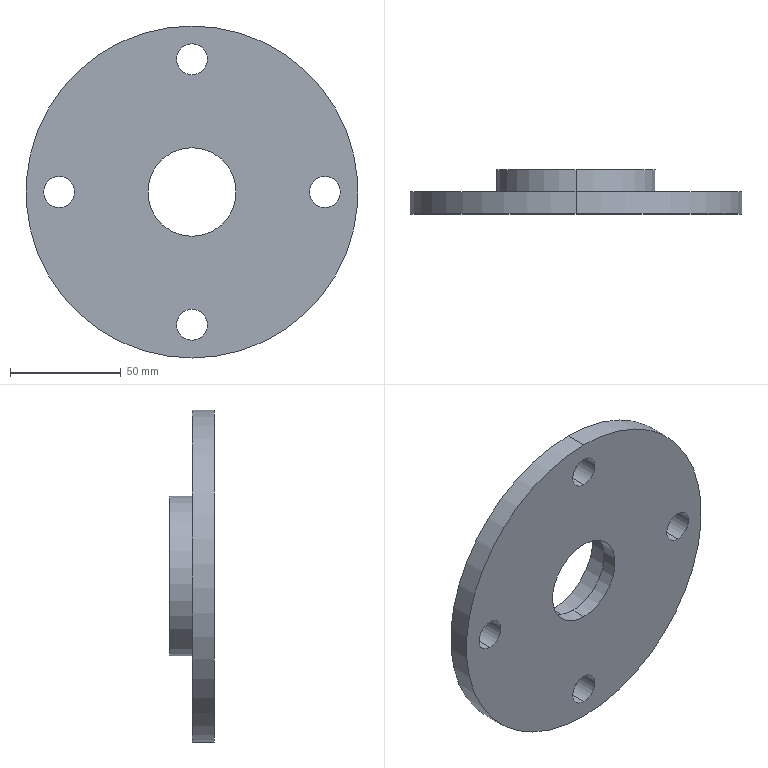Part | SolidWorks | features BaseBody 1 | 1 solid | 20 faces | box 150 x 20 x 150 mm | volume 174867 mm3 | cylinder 16 | plane 4 | commonest cylinder face diameters 14 x8 40 x2 52 x2 72 x2 150 x2
STEP:
#1=CARTESIAN_POINT('',(0.,10.,-75.));
#2=VERTEX_POINT('',#1);
#3=CARTESIAN_POINT('',(0.,10.,75.));
#4=VERTEX_POINT('',#3);
#5=CARTESIAN_POINT('',(0.,10.,0.));
#6=DIRECTION('',(0.,-1.,0.));
#7=DIRECTION('',(0.,0.,-1.));
#8=AXIS2_PLACEMENT_3D('',#5,#6,#7);
#9=CIRCLE('',#8,75.);
#10=EDGE_CURVE('',#2,#4,#9,.T.);
#11=ORIENTED_EDGE('',*,*,#10,.T.);
#12=CARTESIAN_POINT('',(0.,0.,75.));
#13=VERTEX_POINT('',#12);
#14=CARTESIAN_POINT('',(0.,10.,75.));
#15=DIRECTION('',(0.,-1.,0.));
#16=VECTOR('',#15,1000.);
#17=LINE('',#14,#16);
#18=EDGE_CURVE('',#4,#13,#17,.T.);
#19=ORIENTED_EDGE('',*,*,#18,.T.);
#20=CARTESIAN_POINT('',(0.,0.,-75.));
#21=VERTEX_POINT('',#20);
#22=CARTESIAN_POINT('',(0.,0.,0.));
#23=DIRECTION('',(0.,1.,0.));
#24=DIRECTION('',(0.,0.,-1.));
#25=AXIS2_PLACEMENT_3D('',#22,#23,#24);
#26=CIRCLE('',#25,75.);
#27=EDGE_CURVE('',#13,#21,#26,.T.);
#28=ORIENTED_EDGE('',*,*,#27,.T.);
#29=CARTESIAN_POINT('',(0.,10.,-75.));
#30=DIRECTION('',(0.,-1.,0.));
#31=VECTOR('',#30,1000.);
#32=LINE('',#29,#31);
#33=EDGE_CURVE('',#2,#21,#32,.T.);
#34=ORIENTED_EDGE('',*,*,#33,.F.);
#35=EDGE_LOOP('',(#11,#19,#28,#34));
#36=FACE_OUTER_BOUND('',#35,.T.);
#37=CARTESIAN_POINT('',(0.,10.,0.));
#38=DIRECTION('',(0.,-1.,0.));
#39=DIRECTION('',(0.,0.,-1.));
#40=AXIS2_PLACEMENT_3D('',#37,#38,#39);
#41=CYLINDRICAL_SURFACE('',#40,75.);
#42=ADVANCED_FACE('',(#36),#41,.T.);
#43=CARTESIAN_POINT('',(0.,0.,20.));
#44=VERTEX_POINT('',#43);
#45=CARTESIAN_POINT('',(0.,0.,-20.));
#46=VERTEX_POINT('',#45);
#47=CARTESIAN_POINT('',(0.,0.,0.));
#48=DIRECTION('',(0.,-1.,0.));
#49=DIRECTION('',(0.,0.,1.));
#50=AXIS2_PLACEMENT_3D('',#47,#48,#49);
#51=CIRCLE('',#50,20.);
#52=EDGE_CURVE('',#44,#46,#51,.T.);
#53=ORIENTED_EDGE('',*,*,#52,.T.);
#54=CARTESIAN_POINT('',(0.,7.,-20.));
#55=VERTEX_POINT('',#54);
#56=CARTESIAN_POINT('',(0.,0.,-20.));
#57=DIRECTION('',(0.,1.,0.));
#58=VECTOR('',#57,1000.);
#59=LINE('',#56,#58);
#60=EDGE_CURVE('',#46,#55,#59,.T.);
#61=ORIENTED_EDGE('',*,*,#60,.T.);
#62=CARTESIAN_POINT('',(0.,7.,20.));
#63=VERTEX_POINT('',#62);
#64=CARTESIAN_POINT('',(0.,7.,0.));
#65=DIRECTION('',(0.,-1.,0.));
#66=DIRECTION('',(0.,0.,1.));
#67=AXIS2_PLACEMENT_3D('',#64,#65,#66);
#68=CIRCLE('',#67,20.);
#69=EDGE_CURVE('',#63,#55,#68,.T.);
#70=ORIENTED_EDGE('',*,*,#69,.F.);
#71=CARTESIAN_POINT('',(0.,0.,20.));
#72=DIRECTION('',(0.,1.,0.));
#73=VECTOR('',#72,1000.);
#74=LINE('',#71,#73);
#75=EDGE_CURVE('',#44,#63,#74,.T.);
#76=ORIENTED_EDGE('',*,*,#75,.F.);
#77=EDGE_LOOP('',(#53,#61,#70,#76));
#78=FACE_OUTER_BOUND('',#77,.T.);
#79=CARTESIAN_POINT('',(0.,0.,0.));
#80=DIRECTION('',(0.,1.,0.));
#81=DIRECTION('',(0.,0.,1.));
#82=AXIS2_PLACEMENT_3D('',#79,#80,#81);
#83=CYLINDRICAL_SURFACE('',#82,20.);
#84=ADVANCED_FACE('',(#78),#83,.F.);
#85=CARTESIAN_POINT('',(0.,0.,-53.));
#86=VERTEX_POINT('',#85);
#87=CARTESIAN_POINT('',(0.,0.,-67.));
#88=VERTEX_POINT('',#87);
#89=CARTESIAN_POINT('',(0.,0.,-60.));
#90=DIRECTION('',(0.,-1.,0.));
#91=DIRECTION('',(0.,0.,1.));
#92=AXIS2_PLACEMENT_3D('',#89,#90,#91);
#93=CIRCLE('',#92,7.);
#94=EDGE_CURVE('',#86,#88,#93,.T.);
#95=ORIENTED_EDGE('',*,*,#94,.T.);
#96=CARTESIAN_POINT('',(0.,10.,-67.));
#97=VERTEX_POINT('',#96);
#98=CARTESIAN_POINT('',(0.,-3.,-67.));
#99=DIRECTION('',(0.,1.,0.));
#100=VECTOR('',#99,1000.);
#101=LINE('',#98,#100);
#102=EDGE_CURVE('',#88,#97,#101,.T.);
#103=ORIENTED_EDGE('',*,*,#102,.T.);
#104=CARTESIAN_POINT('',(0.,10.,-53.));
#105=VERTEX_POINT('',#104);
#106=CARTESIAN_POINT('',(0.,10.,-60.));
#107=DIRECTION('',(0.,-1.,0.));
#108=DIRECTION('',(0.,0.,1.));
#109=AXIS2_PLACEMENT_3D('',#106,#107,#108);
#110=CIRCLE('',#109,7.);
#111=EDGE_CURVE('',#105,#97,#110,.T.);
#112=ORIENTED_EDGE('',*,*,#111,.F.);
#113=CARTESIAN_POINT('',(0.,-3.,-53.));
#114=DIRECTION('',(0.,1.,0.));
#115=VECTOR('',#114,1000.);
#116=LINE('',#113,#115);
#117=EDGE_CURVE('',#86,#105,#116,.T.);
#118=ORIENTED_EDGE('',*,*,#117,.F.);
#119=EDGE_LOOP('',(#95,#103,#112,#118));
#120=FACE_OUTER_BOUND('',#119,.T.);
#121=CARTESIAN_POINT('',(0.,-3.,-60.));
#122=DIRECTION('',(0.,1.,0.));
#123=DIRECTION('',(0.,0.,1.));
#124=AXIS2_PLACEMENT_3D('',#121,#122,#123);
#125=CYLINDRICAL_SURFACE('',#124,7.);
#126=ADVANCED_FACE('',(#120),#125,.F.);
#127=CARTESIAN_POINT('',(60.,0.,7.));
#128=VERTEX_POINT('',#127);
#129=CARTESIAN_POINT('',(60.,0.,-7.));
#130=VERTEX_POINT('',#129);
#131=CARTESIAN_POINT('',(60.,0.,0.));
#132=DIRECTION('',(0.,-1.,0.));
#133=DIRECTION('',(0.,0.,1.));
#134=AXIS2_PLACEMENT_3D('',#131,#132,#133);
#135=CIRCLE('',#134,7.);
#136=EDGE_CURVE('',#128,#130,#135,.T.);
#137=ORIENTED_EDGE('',*,*,#136,.T.);
#138=CARTESIAN_POINT('',(60.,10.,-7.));
#139=VERTEX_POINT('',#138);
#140=CARTESIAN_POINT('',(60.,-3.,-7.));
#141=DIRECTION('',(0.,1.,0.));
#142=VECTOR('',#141,1000.);
#143=LINE('',#140,#142);
#144=EDGE_CURVE('',#130,#139,#143,.T.);
#145=ORIENTED_EDGE('',*,*,#144,.T.);
#146=CARTESIAN_POINT('',(60.,10.,7.));
#147=VERTEX_POINT('',#146);
#148=CARTESIAN_POINT('',(60.,10.,0.));
#149=DIRECTION('',(0.,-1.,0.));
#150=DIRECTION('',(0.,0.,1.));
#151=AXIS2_PLACEMENT_3D('',#148,#149,#150);
#152=CIRCLE('',#151,7.);
#153=EDGE_CURVE('',#147,#139,#152,.T.);
#154=ORIENTED_EDGE('',*,*,#153,.F.);
#155=CARTESIAN_POINT('',(60.,-3.,7.));
#156=DIRECTION('',(0.,1.,0.));
#157=VECTOR('',#156,1000.);
#158=LINE('',#155,#157);
#159=EDGE_CURVE('',#128,#147,#158,.T.);
#160=ORIENTED_EDGE('',*,*,#159,.F.);
#161=EDGE_LOOP('',(#137,#145,#154,#160));
#162=FACE_OUTER_BOUND('',#161,.T.);
#163=CARTESIAN_POINT('',(60.,-3.,0.));
#164=DIRECTION('',(0.,1.,0.));
#165=DIRECTION('',(0.,0.,1.));
#166=AXIS2_PLACEMENT_3D('',#163,#164,#165);
#167=CYLINDRICAL_SURFACE('',#166,7.);
#168=ADVANCED_FACE('',(#162),#167,.F.);
#169=CARTESIAN_POINT('',(0.,0.,67.));
#170=VERTEX_POINT('',#169);
#171=CARTESIAN_POINT('',(0.,0.,53.));
#172=VERTEX_POINT('',#171);
#173=CARTESIAN_POINT('',(0.,0.,60.));
#174=DIRECTION('',(0.,-1.,0.));
#175=DIRECTION('',(0.,0.,1.));
#176=AXIS2_PLACEMENT_3D('',#173,#174,#175);
#177=CIRCLE('',#176,7.);
#178=EDGE_CURVE('',#170,#172,#177,.T.);
#179=ORIENTED_EDGE('',*,*,#178,.T.);
#180=CARTESIAN_POINT('',(0.,10.,53.));
#181=VERTEX_POINT('',#180);
#182=CARTESIAN_POINT('',(0.,-3.,53.));
#183=DIRECTION('',(0.,1.,0.));
#184=VECTOR('',#183,1000.);
#185=LINE('',#182,#184);
#186=EDGE_CURVE('',#172,#181,#185,.T.);
#187=ORIENTED_EDGE('',*,*,#186,.T.);
#188=CARTESIAN_POINT('',(0.,10.,67.));
#189=VERTEX_POINT('',#188);
#190=CARTESIAN_POINT('',(0.,10.,60.));
#191=DIRECTION('',(0.,-1.,0.));
#192=DIRECTION('',(0.,0.,1.));
#193=AXIS2_PLACEMENT_3D('',#190,#191,#192);
#194=CIRCLE('',#193,7.);
#195=EDGE_CURVE('',#189,#181,#194,.T.);
#196=ORIENTED_EDGE('',*,*,#195,.F.);
#197=CARTESIAN_POINT('',(0.,-3.,67.));
#198=DIRECTION('',(0.,1.,0.));
#199=VECTOR('',#198,1000.);
#200=LINE('',#197,#199);
#201=EDGE_CURVE('',#170,#189,#200,.T.);
#202=ORIENTED_EDGE('',*,*,#201,.F.);
#203=EDGE_LOOP('',(#179,#187,#196,#202));
#204=FACE_OUTER_BOUND('',#203,.T.);
#205=CARTESIAN_POINT('',(0.,-3.,60.));
#206=DIRECTION('',(0.,1.,0.));
#207=DIRECTION('',(0.,0.,1.));
#208=AXIS2_PLACEMENT_3D('',#205,#206,#207);
#209=CYLINDRICAL_SURFACE('',#208,7.);
#210=ADVANCED_FACE('',(#204),#209,.F.);
#211=CARTESIAN_POINT('',(-60.,0.,7.));
#212=VERTEX_POINT('',#211);
#213=CARTESIAN_POINT('',(-60.,0.,-7.));
#214=VERTEX_POINT('',#213);
#215=CARTESIAN_POINT('',(-60.,0.,0.));
#216=DIRECTION('',(0.,-1.,0.));
#217=DIRECTION('',(0.,0.,1.));
#218=AXIS2_PLACEMENT_3D('',#215,#216,#217);
#219=CIRCLE('',#218,7.);
#220=EDGE_CURVE('',#212,#214,#219,.T.);
#221=ORIENTED_EDGE('',*,*,#220,.T.);
#222=CARTESIAN_POINT('',(-60.,10.,-7.));
#223=VERTEX_POINT('',#222);
#224=CARTESIAN_POINT('',(-60.,-3.,-7.));
#225=DIRECTION('',(0.,1.,0.));
#226=VECTOR('',#225,1000.);
#227=LINE('',#224,#226);
#228=EDGE_CURVE('',#214,#223,#227,.T.);
#229=ORIENTED_EDGE('',*,*,#228,.T.);
#230=CARTESIAN_POINT('',(-60.,10.,7.));
#231=VERTEX_POINT('',#230);
#232=CARTESIAN_POINT('',(-60.,10.,0.));
#233=DIRECTION('',(0.,-1.,0.));
#234=DIRECTION('',(0.,0.,1.));
#235=AXIS2_PLACEMENT_3D('',#232,#233,#234);
#236=CIRCLE('',#235,7.);
#237=EDGE_CURVE('',#231,#223,#236,.T.);
#238=ORIENTED_EDGE('',*,*,#237,.F.);
#239=CARTESIAN_POINT('',(-60.,-3.,7.));
#240=DIRECTION('',(0.,1.,0.));
#241=VECTOR('',#240,1000.);
#242=LINE('',#239,#241);
#243=EDGE_CURVE('',#212,#231,#242,.T.);
#244=ORIENTED_EDGE('',*,*,#243,.F.);
#245=EDGE_LOOP('',(#221,#229,#238,#244));
#246=FACE_OUTER_BOUND('',#245,.T.);
#247=CARTESIAN_POINT('',(-60.,-3.,0.));
#248=DIRECTION('',(0.,1.,0.));
#249=DIRECTION('',(0.,0.,1.));
#250=AXIS2_PLACEMENT_3D('',#247,#248,#249);
#251=CYLINDRICAL_SURFACE('',#250,7.);
#252=ADVANCED_FACE('',(#246),#251,.F.);
#253=CARTESIAN_POINT('',(0.,20.,-36.));
#254=VERTEX_POINT('',#253);
#255=CARTESIAN_POINT('',(0.,20.,36.));
#256=VERTEX_POINT('',#255);
#257=CARTESIAN_POINT('',(0.,20.,0.));
#258=DIRECTION('',(0.,-1.,0.));
#259=DIRECTION('',(0.,0.,-1.));
#260=AXIS2_PLACEMENT_3D('',#257,#258,#259);
#261=CIRCLE('',#260,36.);
#262=EDGE_CURVE('',#254,#256,#261,.T.);
#263=ORIENTED_EDGE('',*,*,#262,.T.);
#264=CARTESIAN_POINT('',(0.,10.,36.));
#265=VERTEX_POINT('',#264);
#266=CARTESIAN_POINT('',(0.,20.,36.));
#267=DIRECTION('',(0.,-1.,0.));
#268=VECTOR('',#267,1000.);
#269=LINE('',#266,#268);
#270=EDGE_CURVE('',#256,#265,#269,.T.);
#271=ORIENTED_EDGE('',*,*,#270,.T.);
#272=CARTESIAN_POINT('',(0.,10.,-36.));
#273=VERTEX_POINT('',#272);
#274=CARTESIAN_POINT('',(0.,10.,0.));
#275=DIRECTION('',(0.,-1.,0.));
#276=DIRECTION('',(0.,0.,-1.));
#277=AXIS2_PLACEMENT_3D('',#274,#275,#276);
#278=CIRCLE('',#277,36.);
#279=EDGE_CURVE('',#273,#265,#278,.T.);
#280=ORIENTED_EDGE('',*,*,#279,.F.);
#281=CARTESIAN_POINT('',(0.,20.,-36.));
#282=DIRECTION('',(0.,-1.,0.));
#283=VECTOR('',#282,1000.);
#284=LINE('',#281,#283);
#285=EDGE_CURVE('',#254,#273,#284,.T.);
#286=ORIENTED_EDGE('',*,*,#285,.F.);
#287=EDGE_LOOP('',(#263,#271,#280,#286));
#288=FACE_OUTER_BOUND('',#287,.T.);
#289=CARTESIAN_POINT('',(0.,20.,0.));
#290=DIRECTION('',(0.,-1.,0.));
#291=DIRECTION('',(0.,0.,-1.));
#292=AXIS2_PLACEMENT_3D('',#289,#290,#291);
#293=CYLINDRICAL_SURFACE('',#292,36.);
#294=ADVANCED_FACE('',(#288),#293,.T.);
#295=CARTESIAN_POINT('',(0.,7.,-26.));
#296=VERTEX_POINT('',#295);
#297=CARTESIAN_POINT('',(0.,7.,26.));
#298=VERTEX_POINT('',#297);
#299=CARTESIAN_POINT('',(0.,7.,0.));
#300=DIRECTION('',(0.,1.,0.));
#301=DIRECTION('',(0.,0.,1.));
#302=AXIS2_PLACEMENT_3D('',#299,#300,#301);
#303=CIRCLE('',#302,26.);
#304=EDGE_CURVE('',#296,#298,#303,.T.);
#305=ORIENTED_EDGE('',*,*,#304,.F.);
#306=CARTESIAN_POINT('',(0.,20.,-26.));
#307=VERTEX_POINT('',#306);
#308=CARTESIAN_POINT('',(0.,7.,-26.));
#309=DIRECTION('',(0.,1.,0.));
#310=VECTOR('',#309,1000.);
#311=LINE('',#308,#310);
#312=EDGE_CURVE('',#296,#307,#311,.T.);
#313=ORIENTED_EDGE('',*,*,#312,.T.);
#314=CARTESIAN_POINT('',(0.,20.,26.));
#315=VERTEX_POINT('',#314);
#316=CARTESIAN_POINT('',(0.,20.,0.));
#317=DIRECTION('',(0.,-1.,0.));
#318=DIRECTION('',(0.,0.,1.));
#319=AXIS2_PLACEMENT_3D('',#316,#317,#318);
#320=CIRCLE('',#319,26.);
#321=EDGE_CURVE('',#315,#307,#320,.T.);
#322=ORIENTED_EDGE('',*,*,#321,.F.);
#323=CARTESIAN_POINT('',(0.,7.,26.));
#324=DIRECTION('',(0.,1.,0.));
#325=VECTOR('',#324,1000.);
#326=LINE('',#323,#325);
#327=EDGE_CURVE('',#298,#315,#326,.T.);
#328=ORIENTED_EDGE('',*,*,#327,.F.);
#329=EDGE_LOOP('',(#305,#313,#322,#328));
#330=FACE_OUTER_BOUND('',#329,.T.);
#331=CARTESIAN_POINT('',(0.,7.,0.));
#332=DIRECTION('',(0.,1.,0.));
#333=DIRECTION('',(0.,0.,1.));
#334=AXIS2_PLACEMENT_3D('',#331,#332,#333);
#335=CYLINDRICAL_SURFACE('',#334,26.);
#336=ADVANCED_FACE('',(#330),#335,.F.);
#337=CARTESIAN_POINT('',(0.,0.,0.));
#338=DIRECTION('',(0.,1.,0.));
#339=DIRECTION('',(0.,0.,-1.));
#340=AXIS2_PLACEMENT_3D('',#337,#338,#339);
#341=CIRCLE('',#340,75.);
#342=EDGE_CURVE('',#21,#13,#341,.T.);
#343=ORIENTED_EDGE('',*,*,#342,.F.);
#344=ORIENTED_EDGE('',*,*,#27,.F.);
#345=EDGE_LOOP('',(#343,#344));
#346=FACE_OUTER_BOUND('',#345,.T.);
#347=ORIENTED_EDGE('',*,*,#52,.F.);
#348=CARTESIAN_POINT('',(0.,0.,0.));
#349=DIRECTION('',(0.,-1.,0.));
#350=DIRECTION('',(0.,0.,1.));
#351=AXIS2_PLACEMENT_3D('',#348,#349,#350);
#352=CIRCLE('',#351,20.);
#353=EDGE_CURVE('',#46,#44,#352,.T.);
#354=ORIENTED_EDGE('',*,*,#353,.F.);
#355=EDGE_LOOP('',(#347,#354));
#356=FACE_BOUND('',#355,.T.);
#357=ORIENTED_EDGE('',*,*,#94,.F.);
#358=CARTESIAN_POINT('',(0.,0.,-60.));
#359=DIRECTION('',(0.,-1.,0.));
#360=DIRECTION('',(0.,0.,1.));
#361=AXIS2_PLACEMENT_3D('',#358,#359,#360);
#362=CIRCLE('',#361,7.);
#363=EDGE_CURVE('',#88,#86,#362,.T.);
#364=ORIENTED_EDGE('',*,*,#363,.F.);
#365=EDGE_LOOP('',(#357,#364));
#366=FACE_BOUND('',#365,.T.);
#367=ORIENTED_EDGE('',*,*,#136,.F.);
#368=CARTESIAN_POINT('',(60.,0.,0.));
#369=DIRECTION('',(0.,-1.,0.));
#370=DIRECTION('',(0.,0.,1.));
#371=AXIS2_PLACEMENT_3D('',#368,#369,#370);
#372=CIRCLE('',#371,7.);
#373=EDGE_CURVE('',#130,#128,#372,.T.);
#374=ORIENTED_EDGE('',*,*,#373,.F.);
#375=EDGE_LOOP('',(#367,#374));
#376=FACE_BOUND('',#375,.T.);
#377=ORIENTED_EDGE('',*,*,#178,.F.);
#378=CARTESIAN_POINT('',(0.,0.,60.));
#379=DIRECTION('',(0.,-1.,0.));
#380=DIRECTION('',(0.,0.,1.));
#381=AXIS2_PLACEMENT_3D('',#378,#379,#380);
#382=CIRCLE('',#381,7.);
#383=EDGE_CURVE('',#172,#170,#382,.T.);
#384=ORIENTED_EDGE('',*,*,#383,.F.);
#385=EDGE_LOOP('',(#377,#384));
#386=FACE_BOUND('',#385,.T.);
#387=ORIENTED_EDGE('',*,*,#220,.F.);
#388=CARTESIAN_POINT('',(-60.,0.,0.));
#389=DIRECTION('',(0.,-1.,0.));
#390=DIRECTION('',(0.,0.,1.));
#391=AXIS2_PLACEMENT_3D('',#388,#389,#390);
#392=CIRCLE('',#391,7.);
#393=EDGE_CURVE('',#214,#212,#392,.T.);
#394=ORIENTED_EDGE('',*,*,#393,.F.);
#395=EDGE_LOOP('',(#387,#394));
#396=FACE_BOUND('',#395,.T.);
#397=CARTESIAN_POINT('',(0.,0.,0.));
#398=DIRECTION('',(0.,1.,0.));
#399=DIRECTION('',(0.,0.,1.));
#400=AXIS2_PLACEMENT_3D('',#397,#398,#399);
#401=PLANE('',#400);
#402=ADVANCED_FACE('',(#346,#356,#366,#376,#386,#396),#401,.F.);
#403=ORIENTED_EDGE('',*,*,#18,.F.);
#404=CARTESIAN_POINT('',(0.,10.,0.));
#405=DIRECTION('',(0.,-1.,0.));
#406=DIRECTION('',(0.,0.,-1.));
#407=AXIS2_PLACEMENT_3D('',#404,#405,#406);
#408=CIRCLE('',#407,75.);
#409=EDGE_CURVE('',#4,#2,#408,.T.);
#410=ORIENTED_EDGE('',*,*,#409,.T.);
#411=ORIENTED_EDGE('',*,*,#33,.T.);
#412=ORIENTED_EDGE('',*,*,#342,.T.);
#413=EDGE_LOOP('',(#403,#410,#411,#412));
#414=FACE_OUTER_BOUND('',#413,.T.);
#415=CARTESIAN_POINT('',(0.,10.,0.));
#416=DIRECTION('',(0.,-1.,0.));
#417=DIRECTION('',(0.,0.,-1.));
#418=AXIS2_PLACEMENT_3D('',#415,#416,#417);
#419=CYLINDRICAL_SURFACE('',#418,75.);
#420=ADVANCED_FACE('',(#414),#419,.T.);
#421=ORIENTED_EDGE('',*,*,#60,.F.);
#422=ORIENTED_EDGE('',*,*,#353,.T.);
#423=ORIENTED_EDGE('',*,*,#75,.T.);
#424=CARTESIAN_POINT('',(0.,7.,0.));
#425=DIRECTION('',(0.,-1.,0.));
#426=DIRECTION('',(0.,0.,1.));
#427=AXIS2_PLACEMENT_3D('',#424,#425,#426);
#428=CIRCLE('',#427,20.);
#429=EDGE_CURVE('',#55,#63,#428,.T.);
#430=ORIENTED_EDGE('',*,*,#429,.F.);
#431=EDGE_LOOP('',(#421,#422,#423,#430));
#432=FACE_OUTER_BOUND('',#431,.T.);
#433=CARTESIAN_POINT('',(0.,0.,0.));
#434=DIRECTION('',(0.,1.,0.));
#435=DIRECTION('',(0.,0.,1.));
#436=AXIS2_PLACEMENT_3D('',#433,#434,#435);
#437=CYLINDRICAL_SURFACE('',#436,20.);
#438=ADVANCED_FACE('',(#432),#437,.F.);
#439=ORIENTED_EDGE('',*,*,#102,.F.);
#440=ORIENTED_EDGE('',*,*,#363,.T.);
#441=ORIENTED_EDGE('',*,*,#117,.T.);
#442=CARTESIAN_POINT('',(0.,10.,-60.));
#443=DIRECTION('',(0.,-1.,0.));
#444=DIRECTION('',(0.,0.,1.));
#445=AXIS2_PLACEMENT_3D('',#442,#443,#444);
#446=CIRCLE('',#445,7.);
#447=EDGE_CURVE('',#97,#105,#446,.T.);
#448=ORIENTED_EDGE('',*,*,#447,.F.);
#449=EDGE_LOOP('',(#439,#440,#441,#448));
#450=FACE_OUTER_BOUND('',#449,.T.);
#451=CARTESIAN_POINT('',(0.,-3.,-60.));
#452=DIRECTION('',(0.,1.,0.));
#453=DIRECTION('',(0.,0.,1.));
#454=AXIS2_PLACEMENT_3D('',#451,#452,#453);
#455=CYLINDRICAL_SURFACE('',#454,7.);
#456=ADVANCED_FACE('',(#450),#455,.F.);
#457=ORIENTED_EDGE('',*,*,#144,.F.);
#458=ORIENTED_EDGE('',*,*,#373,.T.);
#459=ORIENTED_EDGE('',*,*,#159,.T.);
#460=CARTESIAN_POINT('',(60.,10.,0.));
#461=DIRECTION('',(0.,-1.,0.));
#462=DIRECTION('',(0.,0.,1.));
#463=AXIS2_PLACEMENT_3D('',#460,#461,#462);
#464=CIRCLE('',#463,7.);
#465=EDGE_CURVE('',#139,#147,#464,.T.);
#466=ORIENTED_EDGE('',*,*,#465,.F.);
#467=EDGE_LOOP('',(#457,#458,#459,#466));
#468=FACE_OUTER_BOUND('',#467,.T.);
#469=CARTESIAN_POINT('',(60.,-3.,0.));
#470=DIRECTION('',(0.,1.,0.));
#471=DIRECTION('',(0.,0.,1.));
#472=AXIS2_PLACEMENT_3D('',#469,#470,#471);
#473=CYLINDRICAL_SURFACE('',#472,7.);
#474=ADVANCED_FACE('',(#468),#473,.F.);
#475=ORIENTED_EDGE('',*,*,#186,.F.);
#476=ORIENTED_EDGE('',*,*,#383,.T.);
#477=ORIENTED_EDGE('',*,*,#201,.T.);
#478=CARTESIAN_POINT('',(0.,10.,60.));
#479=DIRECTION('',(0.,-1.,0.));
#480=DIRECTION('',(0.,0.,1.));
#481=AXIS2_PLACEMENT_3D('',#478,#479,#480);
#482=CIRCLE('',#481,7.);
#483=EDGE_CURVE('',#181,#189,#482,.T.);
#484=ORIENTED_EDGE('',*,*,#483,.F.);
#485=EDGE_LOOP('',(#475,#476,#477,#484));
#486=FACE_OUTER_BOUND('',#485,.T.);
#487=CARTESIAN_POINT('',(0.,-3.,60.));
#488=DIRECTION('',(0.,1.,0.));
#489=DIRECTION('',(0.,0.,1.));
#490=AXIS2_PLACEMENT_3D('',#487,#488,#489);
#491=CYLINDRICAL_SURFACE('',#490,7.);
#492=ADVANCED_FACE('',(#486),#491,.F.);
#493=ORIENTED_EDGE('',*,*,#228,.F.);
#494=ORIENTED_EDGE('',*,*,#393,.T.);
#495=ORIENTED_EDGE('',*,*,#243,.T.);
#496=CARTESIAN_POINT('',(-60.,10.,0.));
#497=DIRECTION('',(0.,-1.,0.));
#498=DIRECTION('',(0.,0.,1.));
#499=AXIS2_PLACEMENT_3D('',#496,#497,#498);
#500=CIRCLE('',#499,7.);
#501=EDGE_CURVE('',#223,#231,#500,.T.);
#502=ORIENTED_EDGE('',*,*,#501,.F.);
#503=EDGE_LOOP('',(#493,#494,#495,#502));
#504=FACE_OUTER_BOUND('',#503,.T.);
#505=CARTESIAN_POINT('',(-60.,-3.,0.));
#506=DIRECTION('',(0.,1.,0.));
#507=DIRECTION('',(0.,0.,1.));
#508=AXIS2_PLACEMENT_3D('',#505,#506,#507);
#509=CYLINDRICAL_SURFACE('',#508,7.);
#510=ADVANCED_FACE('',(#504),#509,.F.);
#511=ORIENTED_EDGE('',*,*,#10,.F.);
#512=ORIENTED_EDGE('',*,*,#409,.F.);
#513=EDGE_LOOP('',(#511,#512));
#514=FACE_OUTER_BOUND('',#513,.T.);
#515=ORIENTED_EDGE('',*,*,#279,.T.);
#516=CARTESIAN_POINT('',(0.,10.,0.));
#517=DIRECTION('',(0.,-1.,0.));
#518=DIRECTION('',(0.,0.,-1.));
#519=AXIS2_PLACEMENT_3D('',#516,#517,#518);
#520=CIRCLE('',#519,36.);
#521=EDGE_CURVE('',#265,#273,#520,.T.);
#522=ORIENTED_EDGE('',*,*,#521,.T.);
#523=EDGE_LOOP('',(#515,#522));
#524=FACE_BOUND('',#523,.T.);
#525=ORIENTED_EDGE('',*,*,#111,.T.);
#526=ORIENTED_EDGE('',*,*,#447,.T.);
#527=EDGE_LOOP('',(#525,#526));
#528=FACE_BOUND('',#527,.T.);
#529=ORIENTED_EDGE('',*,*,#153,.T.);
#530=ORIENTED_EDGE('',*,*,#465,.T.);
#531=EDGE_LOOP('',(#529,#530));
#532=FACE_BOUND('',#531,.T.);
#533=ORIENTED_EDGE('',*,*,#195,.T.);
#534=ORIENTED_EDGE('',*,*,#483,.T.);
#535=EDGE_LOOP('',(#533,#534));
#536=FACE_BOUND('',#535,.T.);
#537=ORIENTED_EDGE('',*,*,#237,.T.);
#538=ORIENTED_EDGE('',*,*,#501,.T.);
#539=EDGE_LOOP('',(#537,#538));
#540=FACE_BOUND('',#539,.T.);
#541=CARTESIAN_POINT('',(0.,10.,0.));
#542=DIRECTION('',(0.,1.,0.));
#543=DIRECTION('',(0.,0.,1.));
#544=AXIS2_PLACEMENT_3D('',#541,#542,#543);
#545=PLANE('',#544);
#546=ADVANCED_FACE('',(#514,#524,#528,#532,#536,#540),#545,.T.);
#547=ORIENTED_EDGE('',*,*,#69,.T.);
#548=ORIENTED_EDGE('',*,*,#429,.T.);
#549=EDGE_LOOP('',(#547,#548));
#550=FACE_BOUND('',#549,.T.);
#551=CARTESIAN_POINT('',(0.,7.,0.));
#552=DIRECTION('',(0.,1.,0.));
#553=DIRECTION('',(0.,0.,1.));
#554=AXIS2_PLACEMENT_3D('',#551,#552,#553);
#555=CIRCLE('',#554,26.);
#556=EDGE_CURVE('',#298,#296,#555,.T.);
#557=ORIENTED_EDGE('',*,*,#556,.T.);
#558=ORIENTED_EDGE('',*,*,#304,.T.);
#559=EDGE_LOOP('',(#557,#558));
#560=FACE_OUTER_BOUND('',#559,.T.);
#561=CARTESIAN_POINT('',(0.,7.,0.));
#562=DIRECTION('',(0.,1.,0.));
#563=DIRECTION('',(0.,0.,1.));
#564=AXIS2_PLACEMENT_3D('',#561,#562,#563);
#565=PLANE('',#564);
#566=ADVANCED_FACE('',(#550,#560),#565,.T.);
#567=ORIENTED_EDGE('',*,*,#270,.F.);
#568=CARTESIAN_POINT('',(0.,20.,0.));
#569=DIRECTION('',(0.,-1.,0.));
#570=DIRECTION('',(0.,0.,-1.));
#571=AXIS2_PLACEMENT_3D('',#568,#569,#570);
#572=CIRCLE('',#571,36.);
#573=EDGE_CURVE('',#256,#254,#572,.T.);
#574=ORIENTED_EDGE('',*,*,#573,.T.);
#575=ORIENTED_EDGE('',*,*,#285,.T.);
#576=ORIENTED_EDGE('',*,*,#521,.F.);
#577=EDGE_LOOP('',(#567,#574,#575,#576));
#578=FACE_OUTER_BOUND('',#577,.T.);
#579=CARTESIAN_POINT('',(0.,20.,0.));
#580=DIRECTION('',(0.,-1.,0.));
#581=DIRECTION('',(0.,0.,-1.));
#582=AXIS2_PLACEMENT_3D('',#579,#580,#581);
#583=CYLINDRICAL_SURFACE('',#582,36.);
#584=ADVANCED_FACE('',(#578),#583,.T.);
#585=ORIENTED_EDGE('',*,*,#312,.F.);
#586=ORIENTED_EDGE('',*,*,#556,.F.);
#587=ORIENTED_EDGE('',*,*,#327,.T.);
#588=CARTESIAN_POINT('',(0.,20.,0.));
#589=DIRECTION('',(0.,-1.,0.));
#590=DIRECTION('',(0.,0.,1.));
#591=AXIS2_PLACEMENT_3D('',#588,#589,#590);
#592=CIRCLE('',#591,26.);
#593=EDGE_CURVE('',#307,#315,#592,.T.);
#594=ORIENTED_EDGE('',*,*,#593,.F.);
#595=EDGE_LOOP('',(#585,#586,#587,#594));
#596=FACE_OUTER_BOUND('',#595,.T.);
#597=CARTESIAN_POINT('',(0.,7.,0.));
#598=DIRECTION('',(0.,1.,0.));
#599=DIRECTION('',(0.,0.,1.));
#600=AXIS2_PLACEMENT_3D('',#597,#598,#599);
#601=CYLINDRICAL_SURFACE('',#600,26.);
#602=ADVANCED_FACE('',(#596),#601,.F.);
#603=ORIENTED_EDGE('',*,*,#262,.F.);
#604=ORIENTED_EDGE('',*,*,#573,.F.);
#605=EDGE_LOOP('',(#603,#604));
#606=FACE_OUTER_BOUND('',#605,.T.);
#607=ORIENTED_EDGE('',*,*,#321,.T.);
#608=ORIENTED_EDGE('',*,*,#593,.T.);
#609=EDGE_LOOP('',(#607,#608));
#610=FACE_BOUND('',#609,.T.);
#611=CARTESIAN_POINT('',(0.,20.,0.));
#612=DIRECTION('',(0.,1.,0.));
#613=DIRECTION('',(0.,0.,1.));
#614=AXIS2_PLACEMENT_3D('',#611,#612,#613);
#615=PLANE('',#614);
#616=ADVANCED_FACE('',(#606,#610),#615,.T.);
#617=CLOSED_SHELL('',(#42,#84,#126,#168,#210,#252,#294,#336,#402,#420,#438,#456,#474,#492,#510,#546,#566,#584,#602,#616));
#618=MANIFOLD_SOLID_BREP('',#617);
#619=CARTESIAN_POINT('',(0.,0.,0.));
#620=DIRECTION('',(0.,0.,1.));
#621=DIRECTION('',(1.,0.,0.));
#622=AXIS2_PLACEMENT_3D('',#619,#620,#621);
#623=(LENGTH_UNIT()NAMED_UNIT(*)SI_UNIT(.MILLI.,.METRE.));
#624=UNCERTAINTY_MEASURE_WITH_UNIT(LENGTH_MEASURE(0.00001),#623,'','');
#625=(NAMED_UNIT(*)PLANE_ANGLE_UNIT()SI_UNIT($,.RADIAN.));
#626=(NAMED_UNIT(*)SI_UNIT($,.STERADIAN.)SOLID_ANGLE_UNIT());
#627=(GEOMETRIC_REPRESENTATION_CONTEXT(3)GLOBAL_UNCERTAINTY_ASSIGNED_CONTEXT((#624))GLOBAL_UNIT_ASSIGNED_CONTEXT((#623,#625,#626))REPRESENTATION_CONTEXT('',''));
#628=ADVANCED_BREP_SHAPE_REPRESENTATION('',(#618,#622),#627);